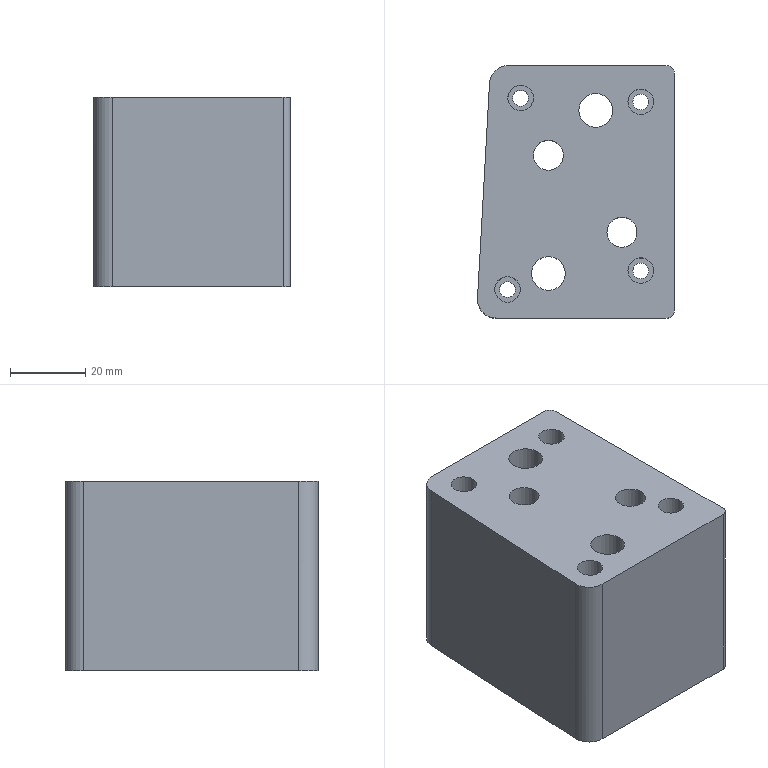Part | NX | features solid 2 | 1 solid | 34 faces | box 52.499 x 67.293 x 50.5 mm | volume 149807 mm3 | cylinder 18 | plane 14 | spline 2 | commonest cylinder face diameters 4.2 x4 6.8 x4 4 x2 8.001 x2 8.5 x2 9 x2
STEP:
#1=CARTESIAN_POINT('',(738.278,22.022,45.));
#2=VERTEX_POINT('',#1);
#3=CARTESIAN_POINT('',(734.878,22.022,45.));
#4=DIRECTION('',(0.,0.,1.));
#5=DIRECTION('',(1.,0.,0.));
#6=AXIS2_PLACEMENT_3D('',#3,#4,#5);
#7=CIRCLE('',#6,3.4);
#8=EDGE_CURVE('',#2,#2,#7,.T.);
#9=ORIENTED_EDGE('',*,*,#8,.F.);
#10=EDGE_LOOP('',(#9));
#11=FACE_BOUND('',#10,.T.);
#12=CARTESIAN_POINT('',(770.278,21.022,45.));
#13=VERTEX_POINT('',#12);
#14=CARTESIAN_POINT('',(766.878,21.022,45.));
#15=DIRECTION('',(0.,0.,1.));
#16=DIRECTION('',(1.,0.,0.));
#17=AXIS2_PLACEMENT_3D('',#14,#15,#16);
#18=CIRCLE('',#17,3.4);
#19=EDGE_CURVE('',#13,#13,#18,.T.);
#20=ORIENTED_EDGE('',*,*,#19,.F.);
#21=EDGE_LOOP('',(#20));
#22=FACE_BOUND('',#21,.T.);
#23=CARTESIAN_POINT('',(770.278,-23.978,45.));
#24=VERTEX_POINT('',#23);
#25=CARTESIAN_POINT('',(766.878,-23.978,45.));
#26=DIRECTION('',(0.,0.,1.));
#27=DIRECTION('',(1.,0.,0.));
#28=AXIS2_PLACEMENT_3D('',#25,#26,#27);
#29=CIRCLE('',#28,3.4);
#30=EDGE_CURVE('',#24,#24,#29,.T.);
#31=ORIENTED_EDGE('',*,*,#30,.F.);
#32=EDGE_LOOP('',(#31));
#33=FACE_BOUND('',#32,.T.);
#34=CARTESIAN_POINT('',(734.778,-28.978,45.));
#35=VERTEX_POINT('',#34);
#36=CARTESIAN_POINT('',(731.378,-28.978,45.));
#37=DIRECTION('',(0.,0.,1.));
#38=DIRECTION('',(1.,0.,0.));
#39=AXIS2_PLACEMENT_3D('',#36,#37,#38);
#40=CIRCLE('',#39,3.4);
#41=EDGE_CURVE('',#35,#35,#40,.T.);
#42=ORIENTED_EDGE('',*,*,#41,.F.);
#43=EDGE_LOOP('',(#42));
#44=FACE_BOUND('',#43,.T.);
#45=CARTESIAN_POINT('',(759.378,18.756,45.));
#46=VERTEX_POINT('',#45);
#47=CARTESIAN_POINT('',(754.878,18.756,45.));
#48=DIRECTION('',(0.,0.,1.));
#49=DIRECTION('',(1.,0.,0.));
#50=AXIS2_PLACEMENT_3D('',#47,#48,#49);
#51=CIRCLE('',#50,4.5);
#52=EDGE_CURVE('',#46,#46,#51,.T.);
#53=ORIENTED_EDGE('',*,*,#52,.F.);
#54=EDGE_LOOP('',(#53));
#55=FACE_BOUND('',#54,.T.);
#56=CARTESIAN_POINT('',(746.284,6.756,45.));
#57=VERTEX_POINT('',#56);
#58=CARTESIAN_POINT('',(742.283,6.756,45.));
#59=DIRECTION('',(0.,0.,1.));
#60=DIRECTION('',(1.,0.,0.));
#61=AXIS2_PLACEMENT_3D('',#58,#59,#60);
#62=CIRCLE('',#61,4.);
#63=EDGE_CURVE('',#57,#57,#62,.T.);
#64=ORIENTED_EDGE('',*,*,#63,.F.);
#65=EDGE_LOOP('',(#64));
#66=FACE_BOUND('',#65,.T.);
#67=CARTESIAN_POINT('',(765.878,-13.727,45.));
#68=VERTEX_POINT('',#67);
#69=CARTESIAN_POINT('',(761.878,-13.727,45.));
#70=DIRECTION('',(0.,0.,1.));
#71=DIRECTION('',(1.,0.,0.));
#72=AXIS2_PLACEMENT_3D('',#69,#70,#71);
#73=CIRCLE('',#72,4.);
#74=EDGE_CURVE('',#68,#68,#73,.T.);
#75=ORIENTED_EDGE('',*,*,#74,.F.);
#76=EDGE_LOOP('',(#75));
#77=FACE_BOUND('',#76,.T.);
#78=CARTESIAN_POINT('',(746.783,-24.727,45.));
#79=VERTEX_POINT('',#78);
#80=CARTESIAN_POINT('',(742.283,-24.727,45.));
#81=DIRECTION('',(0.,0.,1.));
#82=DIRECTION('',(1.,0.,0.));
#83=AXIS2_PLACEMENT_3D('',#80,#81,#82);
#84=CIRCLE('',#83,4.5);
#85=EDGE_CURVE('',#79,#79,#84,.T.);
#86=ORIENTED_EDGE('',*,*,#85,.F.);
#87=EDGE_LOOP('',(#86));
#88=FACE_BOUND('',#87,.T.);
#89=CARTESIAN_POINT('',(723.386,-31.346,45.));
#90=VERTEX_POINT('',#89);
#91=CARTESIAN_POINT('',(726.583,25.947,45.));
#92=VERTEX_POINT('',#91);
#93=CARTESIAN_POINT('',(723.386,-31.346,45.));
#94=DIRECTION('',(0.05572,0.9984,0.));
#95=VECTOR('',#94,1000.);
#96=LINE('',#93,#95);
#97=EDGE_CURVE('',#90,#92,#96,.T.);
#98=ORIENTED_EDGE('',*,*,#97,.F.);
#99=CARTESIAN_POINT('',(728.378,-36.625,45.));
#100=VERTEX_POINT('',#99);
#101=CARTESIAN_POINT('',(728.378,-36.625,45.));
#102=CARTESIAN_POINT('',(727.009,-36.625,45.));
#103=CARTESIAN_POINT('',(724.329,-35.456,45.));
#104=CARTESIAN_POINT('',(723.31,-32.703,45.));
#105=CARTESIAN_POINT('',(723.386,-31.346,45.));
#106=B_SPLINE_CURVE_WITH_KNOTS('',3,(#101,#102,#103,#104,#105),.UNSPECIFIED.,.F.,.F.,(4,1,4),(0.01244,0.01654,0.02065),.UNSPECIFIED.);
#107=EDGE_CURVE('',#100,#90,#106,.T.);
#108=ORIENTED_EDGE('',*,*,#107,.F.);
#109=CARTESIAN_POINT('',(773.878,-36.625,45.));
#110=VERTEX_POINT('',#109);
#111=CARTESIAN_POINT('',(736.409,-36.625,45.));
#112=DIRECTION('',(-1.,0.,0.));
#113=VECTOR('',#112,1000.);
#114=LINE('',#111,#113);
#115=EDGE_CURVE('',#110,#100,#114,.T.);
#116=ORIENTED_EDGE('',*,*,#115,.F.);
#117=CARTESIAN_POINT('',(775.878,-34.625,45.));
#118=VERTEX_POINT('',#117);
#119=CARTESIAN_POINT('',(773.878,-34.625,45.));
#120=DIRECTION('',(0.,0.,1.));
#121=DIRECTION('',(1.,0.,0.));
#122=AXIS2_PLACEMENT_3D('',#119,#120,#121);
#123=CIRCLE('',#122,2.);
#124=EDGE_CURVE('',#118,#110,#123,.F.);
#125=ORIENTED_EDGE('',*,*,#124,.F.);
#126=CARTESIAN_POINT('',(775.878,28.668,45.));
#127=VERTEX_POINT('',#126);
#128=CARTESIAN_POINT('',(775.878,0.7578,45.));
#129=DIRECTION('',(0.,-1.,0.));
#130=VECTOR('',#129,1000.);
#131=LINE('',#128,#130);
#132=EDGE_CURVE('',#127,#118,#131,.T.);
#133=ORIENTED_EDGE('',*,*,#132,.F.);
#134=CARTESIAN_POINT('',(773.878,30.668,45.));
#135=VERTEX_POINT('',#134);
#136=CARTESIAN_POINT('',(773.878,28.668,45.));
#137=DIRECTION('',(0.,0.,1.));
#138=DIRECTION('',(1.,0.,0.));
#139=AXIS2_PLACEMENT_3D('',#136,#137,#138);
#140=CIRCLE('',#139,2.);
#141=EDGE_CURVE('',#135,#127,#140,.F.);
#142=ORIENTED_EDGE('',*,*,#141,.F.);
#143=CARTESIAN_POINT('',(731.575,30.668,45.));
#144=VERTEX_POINT('',#143);
#145=CARTESIAN_POINT('',(731.575,30.668,45.));
#146=DIRECTION('',(1.,-0.000000617,0.));
#147=VECTOR('',#146,1000.);
#148=LINE('',#145,#147);
#149=EDGE_CURVE('',#144,#135,#148,.T.);
#150=ORIENTED_EDGE('',*,*,#149,.F.);
#151=CARTESIAN_POINT('',(726.583,25.947,45.));
#152=CARTESIAN_POINT('',(726.654,27.219,45.));
#153=CARTESIAN_POINT('',(727.799,29.657,45.));
#154=CARTESIAN_POINT('',(730.302,30.668,45.));
#155=CARTESIAN_POINT('',(731.575,30.668,45.));
#156=B_SPLINE_CURVE_WITH_KNOTS('',3,(#151,#152,#153,#154,#155),.UNSPECIFIED.,.F.,.F.,(4,1,4),(0.,0.003767,0.007534),.UNSPECIFIED.);
#157=EDGE_CURVE('',#92,#144,#156,.T.);
#158=ORIENTED_EDGE('',*,*,#157,.F.);
#159=EDGE_LOOP('',(#98,#108,#116,#125,#133,#142,#150,#158));
#160=FACE_BOUND('',#159,.T.);
#161=CARTESIAN_POINT('',(612.,0.,45.));
#162=DIRECTION('',(0.,0.,1.));
#163=DIRECTION('',(1.,0.,0.));
#164=AXIS2_PLACEMENT_3D('',#161,#162,#163);
#165=PLANE('',#164);
#166=ADVANCED_FACE('',(#11,#22,#33,#44,#55,#66,#77,#88,#160),#165,.T.);
#167=CARTESIAN_POINT('',(723.386,-31.346,-5.5));
#168=VERTEX_POINT('',#167);
#169=CARTESIAN_POINT('',(723.386,-31.346,19.75));
#170=DIRECTION('',(0.,0.,-1.));
#171=VECTOR('',#170,1000.);
#172=LINE('',#169,#171);
#173=EDGE_CURVE('',#90,#168,#172,.T.);
#174=ORIENTED_EDGE('',*,*,#173,.F.);
#175=ORIENTED_EDGE('',*,*,#97,.T.);
#176=CARTESIAN_POINT('',(726.583,25.947,-5.5));
#177=VERTEX_POINT('',#176);
#178=CARTESIAN_POINT('',(726.583,25.947,19.75));
#179=DIRECTION('',(0.,0.,-1.));
#180=VECTOR('',#179,1000.);
#181=LINE('',#178,#180);
#182=EDGE_CURVE('',#92,#177,#181,.T.);
#183=ORIENTED_EDGE('',*,*,#182,.T.);
#184=CARTESIAN_POINT('',(723.386,-31.346,-5.5));
#185=DIRECTION('',(0.05572,0.9984,0.));
#186=VECTOR('',#185,1000.);
#187=LINE('',#184,#186);
#188=EDGE_CURVE('',#168,#177,#187,.T.);
#189=ORIENTED_EDGE('',*,*,#188,.F.);
#190=EDGE_LOOP('',(#174,#175,#183,#189));
#191=FACE_BOUND('',#190,.T.);
#192=CARTESIAN_POINT('',(723.386,-31.346,20.));
#193=DIRECTION('',(-0.9984,0.05572,0.));
#194=DIRECTION('',(-0.05572,-0.9984,0.));
#195=AXIS2_PLACEMENT_3D('',#192,#193,#194);
#196=PLANE('',#195);
#197=ADVANCED_FACE('',(#191),#196,.T.);
#198=CARTESIAN_POINT('',(731.575,30.668,-5.5));
#199=VERTEX_POINT('',#198);
#200=CARTESIAN_POINT('',(726.583,25.947,-5.5));
#201=CARTESIAN_POINT('',(726.654,27.219,-5.5));
#202=CARTESIAN_POINT('',(727.799,29.657,-5.5));
#203=CARTESIAN_POINT('',(730.302,30.668,-5.5));
#204=CARTESIAN_POINT('',(731.575,30.668,-5.5));
#205=B_SPLINE_CURVE_WITH_KNOTS('',3,(#200,#201,#202,#203,#204),.UNSPECIFIED.,.F.,.F.,(4,1,4),(0.,0.003767,0.007534),.UNSPECIFIED.);
#206=EDGE_CURVE('',#177,#199,#205,.T.);
#207=ORIENTED_EDGE('',*,*,#206,.F.);
#208=ORIENTED_EDGE('',*,*,#182,.F.);
#209=ORIENTED_EDGE('',*,*,#157,.T.);
#210=CARTESIAN_POINT('',(731.575,30.668,19.75));
#211=DIRECTION('',(0.,0.,-1.));
#212=VECTOR('',#211,1000.);
#213=LINE('',#210,#212);
#214=EDGE_CURVE('',#144,#199,#213,.T.);
#215=ORIENTED_EDGE('',*,*,#214,.T.);
#216=EDGE_LOOP('',(#207,#208,#209,#215));
#217=FACE_BOUND('',#216,.T.);
#218=CARTESIAN_POINT('',(731.575,30.668,45.));
#219=CARTESIAN_POINT('',(731.575,30.668,-5.5));
#220=CARTESIAN_POINT('',(730.31,30.668,45.));
#221=CARTESIAN_POINT('',(730.31,30.668,-5.5));
#222=CARTESIAN_POINT('',(727.797,29.663,45.));
#223=CARTESIAN_POINT('',(727.797,29.663,-5.5));
#224=CARTESIAN_POINT('',(726.653,27.21,45.));
#225=CARTESIAN_POINT('',(726.653,27.21,-5.5));
#226=CARTESIAN_POINT('',(726.583,25.947,45.));
#227=CARTESIAN_POINT('',(726.583,25.947,-5.5));
#228=B_SPLINE_SURFACE_WITH_KNOTS('',3,1,((#218,#219),(#220,#221),(#222,#223),(#224,#225),(#226,#227)),.SURF_OF_LINEAR_EXTRUSION.,.F.,.F.,.F.,(4,1,4),(2,2),(0.,0.5,1.),(0.,1.),.UNSPECIFIED.);
#229=ADVANCED_FACE('',(#217),#228,.F.);
#230=ORIENTED_EDGE('',*,*,#214,.F.);
#231=ORIENTED_EDGE('',*,*,#149,.T.);
#232=CARTESIAN_POINT('',(773.878,30.668,-5.5));
#233=VERTEX_POINT('',#232);
#234=CARTESIAN_POINT('',(773.878,30.668,20.));
#235=DIRECTION('',(0.,0.,1.));
#236=VECTOR('',#235,1000.);
#237=LINE('',#234,#236);
#238=EDGE_CURVE('',#135,#233,#237,.F.);
#239=ORIENTED_EDGE('',*,*,#238,.T.);
#240=CARTESIAN_POINT('',(731.575,30.668,-5.5));
#241=DIRECTION('',(1.,-0.000000617,0.));
#242=VECTOR('',#241,1000.);
#243=LINE('',#240,#242);
#244=EDGE_CURVE('',#199,#233,#243,.T.);
#245=ORIENTED_EDGE('',*,*,#244,.F.);
#246=EDGE_LOOP('',(#230,#231,#239,#245));
#247=FACE_BOUND('',#246,.T.);
#248=CARTESIAN_POINT('',(731.575,30.668,20.));
#249=DIRECTION('',(0.000000617,1.,0.));
#250=DIRECTION('',(-1.,0.000000617,0.));
#251=AXIS2_PLACEMENT_3D('',#248,#249,#250);
#252=PLANE('',#251);
#253=ADVANCED_FACE('',(#247),#252,.T.);
#254=CARTESIAN_POINT('',(775.878,28.668,-5.5));
#255=VERTEX_POINT('',#254);
#256=CARTESIAN_POINT('',(775.878,28.668,0.));
#257=DIRECTION('',(0.,0.,1.));
#258=VECTOR('',#257,1000.);
#259=LINE('',#256,#258);
#260=EDGE_CURVE('',#255,#127,#259,.T.);
#261=ORIENTED_EDGE('',*,*,#260,.T.);
#262=ORIENTED_EDGE('',*,*,#132,.T.);
#263=CARTESIAN_POINT('',(775.878,-34.625,-5.5));
#264=VERTEX_POINT('',#263);
#265=CARTESIAN_POINT('',(775.878,-34.625,0.));
#266=DIRECTION('',(0.,0.,1.));
#267=VECTOR('',#266,1000.);
#268=LINE('',#265,#267);
#269=EDGE_CURVE('',#118,#264,#268,.F.);
#270=ORIENTED_EDGE('',*,*,#269,.T.);
#271=CARTESIAN_POINT('',(775.878,0.7578,-5.5));
#272=DIRECTION('',(0.,-1.,0.));
#273=VECTOR('',#272,1000.);
#274=LINE('',#271,#273);
#275=EDGE_CURVE('',#255,#264,#274,.T.);
#276=ORIENTED_EDGE('',*,*,#275,.F.);
#277=EDGE_LOOP('',(#261,#262,#270,#276));
#278=FACE_BOUND('',#277,.T.);
#279=CARTESIAN_POINT('',(775.878,0.7578,0.));
#280=DIRECTION('',(1.,0.,0.));
#281=DIRECTION('',(0.,0.,-1.));
#282=AXIS2_PLACEMENT_3D('',#279,#280,#281);
#283=PLANE('',#282);
#284=ADVANCED_FACE('',(#278),#283,.T.);
#285=CARTESIAN_POINT('',(773.878,-36.625,-5.5));
#286=VERTEX_POINT('',#285);
#287=CARTESIAN_POINT('',(773.878,-36.625,20.));
#288=DIRECTION('',(0.,0.,1.));
#289=VECTOR('',#288,1000.);
#290=LINE('',#287,#289);
#291=EDGE_CURVE('',#286,#110,#290,.T.);
#292=ORIENTED_EDGE('',*,*,#291,.T.);
#293=ORIENTED_EDGE('',*,*,#115,.T.);
#294=CARTESIAN_POINT('',(728.378,-36.625,-5.5));
#295=VERTEX_POINT('',#294);
#296=CARTESIAN_POINT('',(728.378,-36.625,19.75));
#297=DIRECTION('',(0.,0.,-1.));
#298=VECTOR('',#297,1000.);
#299=LINE('',#296,#298);
#300=EDGE_CURVE('',#100,#295,#299,.T.);
#301=ORIENTED_EDGE('',*,*,#300,.T.);
#302=CARTESIAN_POINT('',(736.409,-36.625,-5.5));
#303=DIRECTION('',(-1.,0.,0.));
#304=VECTOR('',#303,1000.);
#305=LINE('',#302,#304);
#306=EDGE_CURVE('',#286,#295,#305,.T.);
#307=ORIENTED_EDGE('',*,*,#306,.F.);
#308=EDGE_LOOP('',(#292,#293,#301,#307));
#309=FACE_BOUND('',#308,.T.);
#310=CARTESIAN_POINT('',(736.409,-36.625,20.));
#311=DIRECTION('',(0.,-1.,0.));
#312=DIRECTION('',(0.,0.,-1.));
#313=AXIS2_PLACEMENT_3D('',#310,#311,#312);
#314=PLANE('',#313);
#315=ADVANCED_FACE('',(#309),#314,.T.);
#316=ORIENTED_EDGE('',*,*,#300,.F.);
#317=ORIENTED_EDGE('',*,*,#107,.T.);
#318=ORIENTED_EDGE('',*,*,#173,.T.);
#319=CARTESIAN_POINT('',(728.378,-36.625,-5.5));
#320=CARTESIAN_POINT('',(727.033,-36.625,-5.5));
#321=CARTESIAN_POINT('',(724.327,-35.468,-5.5));
#322=CARTESIAN_POINT('',(723.31,-32.699,-5.5));
#323=CARTESIAN_POINT('',(723.386,-31.346,-5.5));
#324=B_SPLINE_CURVE_WITH_KNOTS('',3,(#319,#320,#321,#322,#323),.UNSPECIFIED.,.F.,.F.,(4,1,4),(-0.001722,0.002337,0.006395),.UNSPECIFIED.);
#325=EDGE_CURVE('',#295,#168,#324,.T.);
#326=ORIENTED_EDGE('',*,*,#325,.F.);
#327=EDGE_LOOP('',(#316,#317,#318,#326));
#328=FACE_BOUND('',#327,.T.);
#329=CARTESIAN_POINT('',(728.378,-36.625,45.));
#330=CARTESIAN_POINT('',(728.378,-36.625,-5.5));
#331=CARTESIAN_POINT('',(727.02,-36.625,45.));
#332=CARTESIAN_POINT('',(727.02,-36.625,-5.5));
#333=CARTESIAN_POINT('',(724.326,-35.457,45.));
#334=CARTESIAN_POINT('',(724.326,-35.457,-5.5));
#335=CARTESIAN_POINT('',(723.31,-32.703,45.));
#336=CARTESIAN_POINT('',(723.31,-32.703,-5.5));
#337=CARTESIAN_POINT('',(723.386,-31.346,45.));
#338=CARTESIAN_POINT('',(723.386,-31.346,-5.5));
#339=B_SPLINE_SURFACE_WITH_KNOTS('',3,1,((#329,#330),(#331,#332),(#333,#334),(#335,#336),(#337,#338)),.SURF_OF_LINEAR_EXTRUSION.,.F.,.F.,.F.,(4,1,4),(2,2),(0.,0.5,1.),(0.,1.),.UNSPECIFIED.);
#340=ADVANCED_FACE('',(#328),#339,.T.);
#341=ORIENTED_EDGE('',*,*,#238,.F.);
#342=ORIENTED_EDGE('',*,*,#141,.T.);
#343=ORIENTED_EDGE('',*,*,#260,.F.);
#344=CARTESIAN_POINT('',(773.878,28.668,-5.5));
#345=DIRECTION('',(0.,0.,1.));
#346=DIRECTION('',(1.,0.,0.));
#347=AXIS2_PLACEMENT_3D('',#344,#345,#346);
#348=CIRCLE('',#347,2.);
#349=EDGE_CURVE('',#233,#255,#348,.F.);
#350=ORIENTED_EDGE('',*,*,#349,.F.);
#351=EDGE_LOOP('',(#341,#342,#343,#350));
#352=FACE_BOUND('',#351,.T.);
#353=CARTESIAN_POINT('',(773.878,28.668,0.));
#354=DIRECTION('',(0.,0.,1.));
#355=DIRECTION('',(1.,0.,0.));
#356=AXIS2_PLACEMENT_3D('',#353,#354,#355);
#357=CYLINDRICAL_SURFACE('',#356,2.);
#358=ADVANCED_FACE('',(#352),#357,.T.);
#359=ORIENTED_EDGE('',*,*,#269,.F.);
#360=ORIENTED_EDGE('',*,*,#124,.T.);
#361=ORIENTED_EDGE('',*,*,#291,.F.);
#362=CARTESIAN_POINT('',(773.878,-34.625,-5.5));
#363=DIRECTION('',(0.,0.,1.));
#364=DIRECTION('',(1.,0.,0.));
#365=AXIS2_PLACEMENT_3D('',#362,#363,#364);
#366=CIRCLE('',#365,2.);
#367=EDGE_CURVE('',#264,#286,#366,.F.);
#368=ORIENTED_EDGE('',*,*,#367,.F.);
#369=EDGE_LOOP('',(#359,#360,#361,#368));
#370=FACE_BOUND('',#369,.T.);
#371=CARTESIAN_POINT('',(773.878,-34.625,20.));
#372=DIRECTION('',(0.,0.,1.));
#373=DIRECTION('',(1.,0.,0.));
#374=AXIS2_PLACEMENT_3D('',#371,#372,#373);
#375=CYLINDRICAL_SURFACE('',#374,2.);
#376=ADVANCED_FACE('',(#370),#375,.T.);
#377=CARTESIAN_POINT('',(736.978,22.022,-5.5));
#378=VERTEX_POINT('',#377);
#379=CARTESIAN_POINT('',(734.878,22.022,-5.5));
#380=DIRECTION('',(0.,0.,1.));
#381=DIRECTION('',(1.,0.,0.));
#382=AXIS2_PLACEMENT_3D('',#379,#380,#381);
#383=CIRCLE('',#382,2.1);
#384=EDGE_CURVE('',#378,#378,#383,.T.);
#385=ORIENTED_EDGE('',*,*,#384,.T.);
#386=EDGE_LOOP('',(#385));
#387=FACE_BOUND('',#386,.T.);
#388=CARTESIAN_POINT('',(768.978,21.022,-5.5));
#389=VERTEX_POINT('',#388);
#390=CARTESIAN_POINT('',(766.878,21.022,-5.5));
#391=DIRECTION('',(0.,0.,1.));
#392=DIRECTION('',(1.,0.,0.));
#393=AXIS2_PLACEMENT_3D('',#390,#391,#392);
#394=CIRCLE('',#393,2.1);
#395=EDGE_CURVE('',#389,#389,#394,.T.);
#396=ORIENTED_EDGE('',*,*,#395,.T.);
#397=EDGE_LOOP('',(#396));
#398=FACE_BOUND('',#397,.T.);
#399=CARTESIAN_POINT('',(768.978,-23.978,-5.5));
#400=VERTEX_POINT('',#399);
#401=CARTESIAN_POINT('',(766.878,-23.978,-5.5));
#402=DIRECTION('',(0.,0.,1.));
#403=DIRECTION('',(1.,0.,0.));
#404=AXIS2_PLACEMENT_3D('',#401,#402,#403);
#405=CIRCLE('',#404,2.1);
#406=EDGE_CURVE('',#400,#400,#405,.T.);
#407=ORIENTED_EDGE('',*,*,#406,.T.);
#408=EDGE_LOOP('',(#407));
#409=FACE_BOUND('',#408,.T.);
#410=CARTESIAN_POINT('',(733.478,-28.978,-5.5));
#411=VERTEX_POINT('',#410);
#412=CARTESIAN_POINT('',(731.378,-28.978,-5.5));
#413=DIRECTION('',(0.,0.,1.));
#414=DIRECTION('',(1.,0.,0.));
#415=AXIS2_PLACEMENT_3D('',#412,#413,#414);
#416=CIRCLE('',#415,2.1);
#417=EDGE_CURVE('',#411,#411,#416,.T.);
#418=ORIENTED_EDGE('',*,*,#417,.T.);
#419=EDGE_LOOP('',(#418));
#420=FACE_BOUND('',#419,.T.);
#421=CARTESIAN_POINT('',(762.128,18.756,-5.5));
#422=VERTEX_POINT('',#421);
#423=CARTESIAN_POINT('',(754.878,18.756,-5.5));
#424=DIRECTION('',(0.,0.,1.));
#425=DIRECTION('',(1.,0.,0.));
#426=AXIS2_PLACEMENT_3D('',#423,#424,#425);
#427=CIRCLE('',#426,7.25);
#428=EDGE_CURVE('',#422,#422,#427,.T.);
#429=ORIENTED_EDGE('',*,*,#428,.T.);
#430=EDGE_LOOP('',(#429));
#431=FACE_BOUND('',#430,.T.);
#432=CARTESIAN_POINT('',(746.533,6.756,-5.5));
#433=VERTEX_POINT('',#432);
#434=CARTESIAN_POINT('',(742.283,6.756,-5.5));
#435=DIRECTION('',(0.,0.,1.));
#436=DIRECTION('',(1.,0.,0.));
#437=AXIS2_PLACEMENT_3D('',#434,#435,#436);
#438=CIRCLE('',#437,4.25);
#439=EDGE_CURVE('',#433,#433,#438,.T.);
#440=ORIENTED_EDGE('',*,*,#439,.T.);
#441=EDGE_LOOP('',(#440));
#442=FACE_BOUND('',#441,.T.);
#443=CARTESIAN_POINT('',(766.128,-13.727,-5.5));
#444=VERTEX_POINT('',#443);
#445=CARTESIAN_POINT('',(761.878,-13.727,-5.5));
#446=DIRECTION('',(0.,0.,1.));
#447=DIRECTION('',(1.,0.,0.));
#448=AXIS2_PLACEMENT_3D('',#445,#446,#447);
#449=CIRCLE('',#448,4.25);
#450=EDGE_CURVE('',#444,#444,#449,.T.);
#451=ORIENTED_EDGE('',*,*,#450,.T.);
#452=EDGE_LOOP('',(#451));
#453=FACE_BOUND('',#452,.T.);
#454=CARTESIAN_POINT('',(749.533,-24.727,-5.5));
#455=VERTEX_POINT('',#454);
#456=CARTESIAN_POINT('',(742.283,-24.727,-5.5));
#457=DIRECTION('',(0.,0.,1.));
#458=DIRECTION('',(1.,0.,0.));
#459=AXIS2_PLACEMENT_3D('',#456,#457,#458);
#460=CIRCLE('',#459,7.25);
#461=EDGE_CURVE('',#455,#455,#460,.T.);
#462=ORIENTED_EDGE('',*,*,#461,.T.);
#463=EDGE_LOOP('',(#462));
#464=FACE_BOUND('',#463,.T.);
#465=ORIENTED_EDGE('',*,*,#275,.T.);
#466=ORIENTED_EDGE('',*,*,#367,.T.);
#467=ORIENTED_EDGE('',*,*,#306,.T.);
#468=ORIENTED_EDGE('',*,*,#325,.T.);
#469=ORIENTED_EDGE('',*,*,#188,.T.);
#470=ORIENTED_EDGE('',*,*,#206,.T.);
#471=ORIENTED_EDGE('',*,*,#244,.T.);
#472=ORIENTED_EDGE('',*,*,#349,.T.);
#473=EDGE_LOOP('',(#465,#466,#467,#468,#469,#470,#471,#472));
#474=FACE_BOUND('',#473,.T.);
#475=CARTESIAN_POINT('',(279.237,0.,-5.5));
#476=DIRECTION('',(0.,0.,1.));
#477=DIRECTION('',(1.,0.,0.));
#478=AXIS2_PLACEMENT_3D('',#475,#476,#477);
#479=PLANE('',#478);
#480=ADVANCED_FACE('',(#387,#398,#409,#420,#431,#442,#453,#464,#474),#479,.F.);
#481=ORIENTED_EDGE('',*,*,#85,.T.);
#482=EDGE_LOOP('',(#481));
#483=FACE_BOUND('',#482,.T.);
#484=CARTESIAN_POINT('',(746.783,-24.727,20.));
#485=VERTEX_POINT('',#484);
#486=CARTESIAN_POINT('',(742.283,-24.727,20.));
#487=DIRECTION('',(0.,0.,1.));
#488=DIRECTION('',(1.,0.,0.));
#489=AXIS2_PLACEMENT_3D('',#486,#487,#488);
#490=CIRCLE('',#489,4.5);
#491=EDGE_CURVE('',#485,#485,#490,.T.);
#492=ORIENTED_EDGE('',*,*,#491,.F.);
#493=EDGE_LOOP('',(#492));
#494=FACE_BOUND('',#493,.T.);
#495=CARTESIAN_POINT('',(742.283,-24.727,-10.5));
#496=DIRECTION('',(0.,0.,1.));
#497=DIRECTION('',(1.,0.,0.));
#498=AXIS2_PLACEMENT_3D('',#495,#496,#497);
#499=CYLINDRICAL_SURFACE('',#498,4.5);
#500=ADVANCED_FACE('',(#483,#494),#499,.F.);
#501=ORIENTED_EDGE('',*,*,#491,.T.);
#502=EDGE_LOOP('',(#501));
#503=FACE_BOUND('',#502,.T.);
#504=CARTESIAN_POINT('',(749.533,-24.727,20.));
#505=VERTEX_POINT('',#504);
#506=CARTESIAN_POINT('',(742.283,-24.727,20.));
#507=DIRECTION('',(0.,0.,-1.));
#508=DIRECTION('',(1.,0.,0.));
#509=AXIS2_PLACEMENT_3D('',#506,#507,#508);
#510=CIRCLE('',#509,7.25);
#511=EDGE_CURVE('',#505,#505,#510,.F.);
#512=ORIENTED_EDGE('',*,*,#511,.F.);
#513=EDGE_LOOP('',(#512));
#514=FACE_BOUND('',#513,.T.);
#515=CARTESIAN_POINT('',(742.283,-24.727,20.));
#516=DIRECTION('',(0.,0.,1.));
#517=DIRECTION('',(1.,0.,0.));
#518=AXIS2_PLACEMENT_3D('',#515,#516,#517);
#519=PLANE('',#518);
#520=ADVANCED_FACE('',(#503,#514),#519,.F.);
#521=ORIENTED_EDGE('',*,*,#511,.T.);
#522=EDGE_LOOP('',(#521));
#523=FACE_BOUND('',#522,.T.);
#524=ORIENTED_EDGE('',*,*,#461,.F.);
#525=EDGE_LOOP('',(#524));
#526=FACE_BOUND('',#525,.T.);
#527=CARTESIAN_POINT('',(742.283,-24.727,-5.5));
#528=DIRECTION('',(0.,0.,1.));
#529=DIRECTION('',(1.,0.,0.));
#530=AXIS2_PLACEMENT_3D('',#527,#528,#529);
#531=CYLINDRICAL_SURFACE('',#530,7.25);
#532=ADVANCED_FACE('',(#523,#526),#531,.F.);
#533=CARTESIAN_POINT('',(766.128,-13.727,21.));
#534=VERTEX_POINT('',#533);
#535=CARTESIAN_POINT('',(761.878,-13.727,21.));
#536=DIRECTION('',(0.,0.,1.));
#537=DIRECTION('',(1.,0.,0.));
#538=AXIS2_PLACEMENT_3D('',#535,#536,#537);
#539=CIRCLE('',#538,4.25);
#540=EDGE_CURVE('',#534,#534,#539,.T.);
#541=ORIENTED_EDGE('',*,*,#540,.T.);
#542=EDGE_LOOP('',(#541));
#543=FACE_BOUND('',#542,.T.);
#544=ORIENTED_EDGE('',*,*,#450,.F.);
#545=EDGE_LOOP('',(#544));
#546=FACE_BOUND('',#545,.T.);
#547=CARTESIAN_POINT('',(761.878,-13.727,-10.5));
#548=DIRECTION('',(0.,0.,1.));
#549=DIRECTION('',(1.,0.,0.));
#550=AXIS2_PLACEMENT_3D('',#547,#548,#549);
#551=CYLINDRICAL_SURFACE('',#550,4.25);
#552=ADVANCED_FACE('',(#543,#546),#551,.F.);
#553=ORIENTED_EDGE('',*,*,#74,.T.);
#554=EDGE_LOOP('',(#553));
#555=FACE_BOUND('',#554,.T.);
#556=CARTESIAN_POINT('',(765.878,-13.727,21.));
#557=VERTEX_POINT('',#556);
#558=CARTESIAN_POINT('',(761.878,-13.727,21.));
#559=DIRECTION('',(0.,0.,1.));
#560=DIRECTION('',(1.,0.,0.));
#561=AXIS2_PLACEMENT_3D('',#558,#559,#560);
#562=CIRCLE('',#561,4.);
#563=EDGE_CURVE('',#557,#557,#562,.T.);
#564=ORIENTED_EDGE('',*,*,#563,.F.);
#565=EDGE_LOOP('',(#564));
#566=FACE_BOUND('',#565,.T.);
#567=CARTESIAN_POINT('',(761.878,-13.727,-10.5));
#568=DIRECTION('',(0.,0.,1.));
#569=DIRECTION('',(1.,0.,0.));
#570=AXIS2_PLACEMENT_3D('',#567,#568,#569);
#571=CYLINDRICAL_SURFACE('',#570,4.);
#572=ADVANCED_FACE('',(#555,#566),#571,.F.);
#573=ORIENTED_EDGE('',*,*,#563,.T.);
#574=EDGE_LOOP('',(#573));
#575=FACE_BOUND('',#574,.T.);
#576=ORIENTED_EDGE('',*,*,#540,.F.);
#577=EDGE_LOOP('',(#576));
#578=FACE_BOUND('',#577,.T.);
#579=CARTESIAN_POINT('',(761.878,-13.727,21.));
#580=DIRECTION('',(0.,0.,1.));
#581=DIRECTION('',(1.,0.,0.));
#582=AXIS2_PLACEMENT_3D('',#579,#580,#581);
#583=PLANE('',#582);
#584=ADVANCED_FACE('',(#575,#578),#583,.F.);
#585=CARTESIAN_POINT('',(746.533,6.756,21.));
#586=VERTEX_POINT('',#585);
#587=CARTESIAN_POINT('',(742.283,6.756,21.));
#588=DIRECTION('',(0.,0.,1.));
#589=DIRECTION('',(1.,0.,0.));
#590=AXIS2_PLACEMENT_3D('',#587,#588,#589);
#591=CIRCLE('',#590,4.25);
#592=EDGE_CURVE('',#586,#586,#591,.T.);
#593=ORIENTED_EDGE('',*,*,#592,.T.);
#594=EDGE_LOOP('',(#593));
#595=FACE_BOUND('',#594,.T.);
#596=ORIENTED_EDGE('',*,*,#439,.F.);
#597=EDGE_LOOP('',(#596));
#598=FACE_BOUND('',#597,.T.);
#599=CARTESIAN_POINT('',(742.283,6.756,-10.5));
#600=DIRECTION('',(0.,0.,1.));
#601=DIRECTION('',(1.,0.,0.));
#602=AXIS2_PLACEMENT_3D('',#599,#600,#601);
#603=CYLINDRICAL_SURFACE('',#602,4.25);
#604=ADVANCED_FACE('',(#595,#598),#603,.F.);
#605=ORIENTED_EDGE('',*,*,#63,.T.);
#606=EDGE_LOOP('',(#605));
#607=FACE_BOUND('',#606,.T.);
#608=CARTESIAN_POINT('',(746.284,6.756,21.));
#609=VERTEX_POINT('',#608);
#610=CARTESIAN_POINT('',(742.283,6.756,21.));
#611=DIRECTION('',(0.,0.,1.));
#612=DIRECTION('',(1.,0.,0.));
#613=AXIS2_PLACEMENT_3D('',#610,#611,#612);
#614=CIRCLE('',#613,4.);
#615=EDGE_CURVE('',#609,#609,#614,.T.);
#616=ORIENTED_EDGE('',*,*,#615,.F.);
#617=EDGE_LOOP('',(#616));
#618=FACE_BOUND('',#617,.T.);
#619=CARTESIAN_POINT('',(742.283,6.756,-10.5));
#620=DIRECTION('',(0.,0.,1.));
#621=DIRECTION('',(1.,0.,0.));
#622=AXIS2_PLACEMENT_3D('',#619,#620,#621);
#623=CYLINDRICAL_SURFACE('',#622,4.);
#624=ADVANCED_FACE('',(#607,#618),#623,.F.);
#625=ORIENTED_EDGE('',*,*,#615,.T.);
#626=EDGE_LOOP('',(#625));
#627=FACE_BOUND('',#626,.T.);
#628=ORIENTED_EDGE('',*,*,#592,.F.);
#629=EDGE_LOOP('',(#628));
#630=FACE_BOUND('',#629,.T.);
#631=CARTESIAN_POINT('',(742.283,6.756,21.));
#632=DIRECTION('',(0.,0.,1.));
#633=DIRECTION('',(1.,0.,0.));
#634=AXIS2_PLACEMENT_3D('',#631,#632,#633);
#635=PLANE('',#634);
#636=ADVANCED_FACE('',(#627,#630),#635,.F.);
#637=ORIENTED_EDGE('',*,*,#52,.T.);
#638=EDGE_LOOP('',(#637));
#639=FACE_BOUND('',#638,.T.);
#640=CARTESIAN_POINT('',(759.378,18.756,20.));
#641=VERTEX_POINT('',#640);
#642=CARTESIAN_POINT('',(754.878,18.756,20.));
#643=DIRECTION('',(0.,0.,1.));
#644=DIRECTION('',(1.,0.,0.));
#645=AXIS2_PLACEMENT_3D('',#642,#643,#644);
#646=CIRCLE('',#645,4.5);
#647=EDGE_CURVE('',#641,#641,#646,.T.);
#648=ORIENTED_EDGE('',*,*,#647,.F.);
#649=EDGE_LOOP('',(#648));
#650=FACE_BOUND('',#649,.T.);
#651=CARTESIAN_POINT('',(754.878,18.756,-10.5));
#652=DIRECTION('',(0.,0.,1.));
#653=DIRECTION('',(1.,0.,0.));
#654=AXIS2_PLACEMENT_3D('',#651,#652,#653);
#655=CYLINDRICAL_SURFACE('',#654,4.5);
#656=ADVANCED_FACE('',(#639,#650),#655,.F.);
#657=ORIENTED_EDGE('',*,*,#647,.T.);
#658=EDGE_LOOP('',(#657));
#659=FACE_BOUND('',#658,.T.);
#660=CARTESIAN_POINT('',(762.128,18.756,20.));
#661=VERTEX_POINT('',#660);
#662=CARTESIAN_POINT('',(754.878,18.756,20.));
#663=DIRECTION('',(0.,0.,-1.));
#664=DIRECTION('',(1.,0.,0.));
#665=AXIS2_PLACEMENT_3D('',#662,#663,#664);
#666=CIRCLE('',#665,7.25);
#667=EDGE_CURVE('',#661,#661,#666,.F.);
#668=ORIENTED_EDGE('',*,*,#667,.F.);
#669=EDGE_LOOP('',(#668));
#670=FACE_BOUND('',#669,.T.);
#671=CARTESIAN_POINT('',(754.878,18.756,20.));
#672=DIRECTION('',(0.,0.,1.));
#673=DIRECTION('',(1.,0.,0.));
#674=AXIS2_PLACEMENT_3D('',#671,#672,#673);
#675=PLANE('',#674);
#676=ADVANCED_FACE('',(#659,#670),#675,.F.);
#677=ORIENTED_EDGE('',*,*,#667,.T.);
#678=EDGE_LOOP('',(#677));
#679=FACE_BOUND('',#678,.T.);
#680=ORIENTED_EDGE('',*,*,#428,.F.);
#681=EDGE_LOOP('',(#680));
#682=FACE_BOUND('',#681,.T.);
#683=CARTESIAN_POINT('',(754.878,18.756,-5.5));
#684=DIRECTION('',(0.,0.,1.));
#685=DIRECTION('',(1.,0.,0.));
#686=AXIS2_PLACEMENT_3D('',#683,#684,#685);
#687=CYLINDRICAL_SURFACE('',#686,7.25);
#688=ADVANCED_FACE('',(#679,#682),#687,.F.);
#689=CARTESIAN_POINT('',(729.278,-28.978,14.5));
#690=VERTEX_POINT('',#689);
#691=CARTESIAN_POINT('',(731.378,-28.978,14.5));
#692=DIRECTION('',(0.,0.,-1.));
#693=DIRECTION('',(-1.,0.,0.));
#694=AXIS2_PLACEMENT_3D('',#691,#692,#693);
#695=CIRCLE('',#694,2.1);
#696=EDGE_CURVE('',#690,#690,#695,.T.);
#697=ORIENTED_EDGE('',*,*,#696,.F.);
#698=EDGE_LOOP('',(#697));
#699=FACE_BOUND('',#698,.T.);
#700=ORIENTED_EDGE('',*,*,#417,.F.);
#701=EDGE_LOOP('',(#700));
#702=FACE_BOUND('',#701,.T.);
#703=CARTESIAN_POINT('',(731.378,-28.978,32.5));
#704=DIRECTION('',(0.,0.,-1.));
#705=DIRECTION('',(1.,0.,0.));
#706=AXIS2_PLACEMENT_3D('',#703,#704,#705);
#707=CYLINDRICAL_SURFACE('',#706,2.1);
#708=ADVANCED_FACE('',(#699,#702),#707,.F.);
#709=ORIENTED_EDGE('',*,*,#696,.T.);
#710=EDGE_LOOP('',(#709));
#711=FACE_BOUND('',#710,.T.);
#712=CARTESIAN_POINT('',(727.978,-28.978,14.5));
#713=VERTEX_POINT('',#712);
#714=CARTESIAN_POINT('',(731.378,-28.978,14.5));
#715=DIRECTION('',(0.,0.,-1.));
#716=DIRECTION('',(-1.,0.,0.));
#717=AXIS2_PLACEMENT_3D('',#714,#715,#716);
#718=CIRCLE('',#717,3.4);
#719=EDGE_CURVE('',#713,#713,#718,.T.);
#720=ORIENTED_EDGE('',*,*,#719,.F.);
#721=EDGE_LOOP('',(#720));
#722=FACE_BOUND('',#721,.T.);
#723=CARTESIAN_POINT('',(731.378,-28.978,14.5));
#724=DIRECTION('',(0.,0.,-1.));
#725=DIRECTION('',(-1.,0.,0.));
#726=AXIS2_PLACEMENT_3D('',#723,#724,#725);
#727=PLANE('',#726);
#728=ADVANCED_FACE('',(#711,#722),#727,.F.);
#729=ORIENTED_EDGE('',*,*,#41,.T.);
#730=EDGE_LOOP('',(#729));
#731=FACE_BOUND('',#730,.T.);
#732=ORIENTED_EDGE('',*,*,#719,.T.);
#733=EDGE_LOOP('',(#732));
#734=FACE_BOUND('',#733,.T.);
#735=CARTESIAN_POINT('',(731.378,-28.978,29.5));
#736=DIRECTION('',(0.,0.,1.));
#737=DIRECTION('',(1.,0.,0.));
#738=AXIS2_PLACEMENT_3D('',#735,#736,#737);
#739=CYLINDRICAL_SURFACE('',#738,3.4);
#740=ADVANCED_FACE('',(#731,#734),#739,.F.);
#741=CARTESIAN_POINT('',(764.778,-23.978,14.5));
#742=VERTEX_POINT('',#741);
#743=CARTESIAN_POINT('',(766.878,-23.978,14.5));
#744=DIRECTION('',(0.,0.,-1.));
#745=DIRECTION('',(-1.,0.,0.));
#746=AXIS2_PLACEMENT_3D('',#743,#744,#745);
#747=CIRCLE('',#746,2.1);
#748=EDGE_CURVE('',#742,#742,#747,.T.);
#749=ORIENTED_EDGE('',*,*,#748,.F.);
#750=EDGE_LOOP('',(#749));
#751=FACE_BOUND('',#750,.T.);
#752=ORIENTED_EDGE('',*,*,#406,.F.);
#753=EDGE_LOOP('',(#752));
#754=FACE_BOUND('',#753,.T.);
#755=CARTESIAN_POINT('',(766.878,-23.978,32.5));
#756=DIRECTION('',(0.,0.,-1.));
#757=DIRECTION('',(1.,0.,0.));
#758=AXIS2_PLACEMENT_3D('',#755,#756,#757);
#759=CYLINDRICAL_SURFACE('',#758,2.1);
#760=ADVANCED_FACE('',(#751,#754),#759,.F.);
#761=ORIENTED_EDGE('',*,*,#748,.T.);
#762=EDGE_LOOP('',(#761));
#763=FACE_BOUND('',#762,.T.);
#764=CARTESIAN_POINT('',(763.478,-23.978,14.5));
#765=VERTEX_POINT('',#764);
#766=CARTESIAN_POINT('',(766.878,-23.978,14.5));
#767=DIRECTION('',(0.,0.,-1.));
#768=DIRECTION('',(-1.,0.,0.));
#769=AXIS2_PLACEMENT_3D('',#766,#767,#768);
#770=CIRCLE('',#769,3.4);
#771=EDGE_CURVE('',#765,#765,#770,.T.);
#772=ORIENTED_EDGE('',*,*,#771,.F.);
#773=EDGE_LOOP('',(#772));
#774=FACE_BOUND('',#773,.T.);
#775=CARTESIAN_POINT('',(766.878,-23.978,14.5));
#776=DIRECTION('',(0.,0.,-1.));
#777=DIRECTION('',(-1.,0.,0.));
#778=AXIS2_PLACEMENT_3D('',#775,#776,#777);
#779=PLANE('',#778);
#780=ADVANCED_FACE('',(#763,#774),#779,.F.);
#781=ORIENTED_EDGE('',*,*,#30,.T.);
#782=EDGE_LOOP('',(#781));
#783=FACE_BOUND('',#782,.T.);
#784=ORIENTED_EDGE('',*,*,#771,.T.);
#785=EDGE_LOOP('',(#784));
#786=FACE_BOUND('',#785,.T.);
#787=CARTESIAN_POINT('',(766.878,-23.978,29.5));
#788=DIRECTION('',(0.,0.,1.));
#789=DIRECTION('',(1.,0.,0.));
#790=AXIS2_PLACEMENT_3D('',#787,#788,#789);
#791=CYLINDRICAL_SURFACE('',#790,3.4);
#792=ADVANCED_FACE('',(#783,#786),#791,.F.);
#793=CARTESIAN_POINT('',(764.778,21.022,14.5));
#794=VERTEX_POINT('',#793);
#795=CARTESIAN_POINT('',(766.878,21.022,14.5));
#796=DIRECTION('',(0.,0.,-1.));
#797=DIRECTION('',(-1.,0.,0.));
#798=AXIS2_PLACEMENT_3D('',#795,#796,#797);
#799=CIRCLE('',#798,2.1);
#800=EDGE_CURVE('',#794,#794,#799,.T.);
#801=ORIENTED_EDGE('',*,*,#800,.F.);
#802=EDGE_LOOP('',(#801));
#803=FACE_BOUND('',#802,.T.);
#804=ORIENTED_EDGE('',*,*,#395,.F.);
#805=EDGE_LOOP('',(#804));
#806=FACE_BOUND('',#805,.T.);
#807=CARTESIAN_POINT('',(766.878,21.022,32.5));
#808=DIRECTION('',(0.,0.,-1.));
#809=DIRECTION('',(1.,0.,0.));
#810=AXIS2_PLACEMENT_3D('',#807,#808,#809);
#811=CYLINDRICAL_SURFACE('',#810,2.1);
#812=ADVANCED_FACE('',(#803,#806),#811,.F.);
#813=ORIENTED_EDGE('',*,*,#800,.T.);
#814=EDGE_LOOP('',(#813));
#815=FACE_BOUND('',#814,.T.);
#816=CARTESIAN_POINT('',(763.478,21.022,14.5));
#817=VERTEX_POINT('',#816);
#818=CARTESIAN_POINT('',(766.878,21.022,14.5));
#819=DIRECTION('',(0.,0.,-1.));
#820=DIRECTION('',(-1.,0.,0.));
#821=AXIS2_PLACEMENT_3D('',#818,#819,#820);
#822=CIRCLE('',#821,3.4);
#823=EDGE_CURVE('',#817,#817,#822,.T.);
#824=ORIENTED_EDGE('',*,*,#823,.F.);
#825=EDGE_LOOP('',(#824));
#826=FACE_BOUND('',#825,.T.);
#827=CARTESIAN_POINT('',(766.878,21.022,14.5));
#828=DIRECTION('',(0.,0.,-1.));
#829=DIRECTION('',(-1.,0.,0.));
#830=AXIS2_PLACEMENT_3D('',#827,#828,#829);
#831=PLANE('',#830);
#832=ADVANCED_FACE('',(#815,#826),#831,.F.);
#833=ORIENTED_EDGE('',*,*,#19,.T.);
#834=EDGE_LOOP('',(#833));
#835=FACE_BOUND('',#834,.T.);
#836=ORIENTED_EDGE('',*,*,#823,.T.);
#837=EDGE_LOOP('',(#836));
#838=FACE_BOUND('',#837,.T.);
#839=CARTESIAN_POINT('',(766.878,21.022,29.5));
#840=DIRECTION('',(0.,0.,1.));
#841=DIRECTION('',(1.,0.,0.));
#842=AXIS2_PLACEMENT_3D('',#839,#840,#841);
#843=CYLINDRICAL_SURFACE('',#842,3.4);
#844=ADVANCED_FACE('',(#835,#838),#843,.F.);
#845=CARTESIAN_POINT('',(732.778,22.022,14.5));
#846=VERTEX_POINT('',#845);
#847=CARTESIAN_POINT('',(734.878,22.022,14.5));
#848=DIRECTION('',(0.,0.,-1.));
#849=DIRECTION('',(-1.,0.,0.));
#850=AXIS2_PLACEMENT_3D('',#847,#848,#849);
#851=CIRCLE('',#850,2.1);
#852=EDGE_CURVE('',#846,#846,#851,.T.);
#853=ORIENTED_EDGE('',*,*,#852,.F.);
#854=EDGE_LOOP('',(#853));
#855=FACE_BOUND('',#854,.T.);
#856=ORIENTED_EDGE('',*,*,#384,.F.);
#857=EDGE_LOOP('',(#856));
#858=FACE_BOUND('',#857,.T.);
#859=CARTESIAN_POINT('',(734.878,22.022,32.5));
#860=DIRECTION('',(0.,0.,-1.));
#861=DIRECTION('',(1.,0.,0.));
#862=AXIS2_PLACEMENT_3D('',#859,#860,#861);
#863=CYLINDRICAL_SURFACE('',#862,2.1);
#864=ADVANCED_FACE('',(#855,#858),#863,.F.);
#865=ORIENTED_EDGE('',*,*,#852,.T.);
#866=EDGE_LOOP('',(#865));
#867=FACE_BOUND('',#866,.T.);
#868=CARTESIAN_POINT('',(731.478,22.022,14.5));
#869=VERTEX_POINT('',#868);
#870=CARTESIAN_POINT('',(734.878,22.022,14.5));
#871=DIRECTION('',(0.,0.,-1.));
#872=DIRECTION('',(-1.,0.,0.));
#873=AXIS2_PLACEMENT_3D('',#870,#871,#872);
#874=CIRCLE('',#873,3.4);
#875=EDGE_CURVE('',#869,#869,#874,.T.);
#876=ORIENTED_EDGE('',*,*,#875,.F.);
#877=EDGE_LOOP('',(#876));
#878=FACE_BOUND('',#877,.T.);
#879=CARTESIAN_POINT('',(734.878,22.022,14.5));
#880=DIRECTION('',(0.,0.,-1.));
#881=DIRECTION('',(-1.,0.,0.));
#882=AXIS2_PLACEMENT_3D('',#879,#880,#881);
#883=PLANE('',#882);
#884=ADVANCED_FACE('',(#867,#878),#883,.F.);
#885=ORIENTED_EDGE('',*,*,#8,.T.);
#886=EDGE_LOOP('',(#885));
#887=FACE_BOUND('',#886,.T.);
#888=ORIENTED_EDGE('',*,*,#875,.T.);
#889=EDGE_LOOP('',(#888));
#890=FACE_BOUND('',#889,.T.);
#891=CARTESIAN_POINT('',(734.878,22.022,29.5));
#892=DIRECTION('',(0.,0.,1.));
#893=DIRECTION('',(1.,0.,0.));
#894=AXIS2_PLACEMENT_3D('',#891,#892,#893);
#895=CYLINDRICAL_SURFACE('',#894,3.4);
#896=ADVANCED_FACE('',(#887,#890),#895,.F.);
#897=CLOSED_SHELL('',(#166,#197,#229,#253,#284,#315,#340,#358,#376,#480,#500,#520,#532,#552,#572,#584,#604,#624,#636,#656,#676,#688,#708,#728,#740,#760,#780,#792,#812,#832,#844,#864,#884,#896));
#898=MANIFOLD_SOLID_BREP('',#897);
#899=(LENGTH_UNIT()NAMED_UNIT(*)SI_UNIT(.MILLI.,.METRE.));
#900=UNCERTAINTY_MEASURE_WITH_UNIT(LENGTH_MEASURE(0.0508),#899,'','');
#901=(NAMED_UNIT(*)PLANE_ANGLE_UNIT()SI_UNIT($,.RADIAN.));
#902=(NAMED_UNIT(*)SI_UNIT($,.STERADIAN.)SOLID_ANGLE_UNIT());
#903=(GEOMETRIC_REPRESENTATION_CONTEXT(3)GLOBAL_UNCERTAINTY_ASSIGNED_CONTEXT((#900))GLOBAL_UNIT_ASSIGNED_CONTEXT((#899,#901,#902))REPRESENTATION_CONTEXT('',''));
#904=ADVANCED_BREP_SHAPE_REPRESENTATION('',(#898),#903);